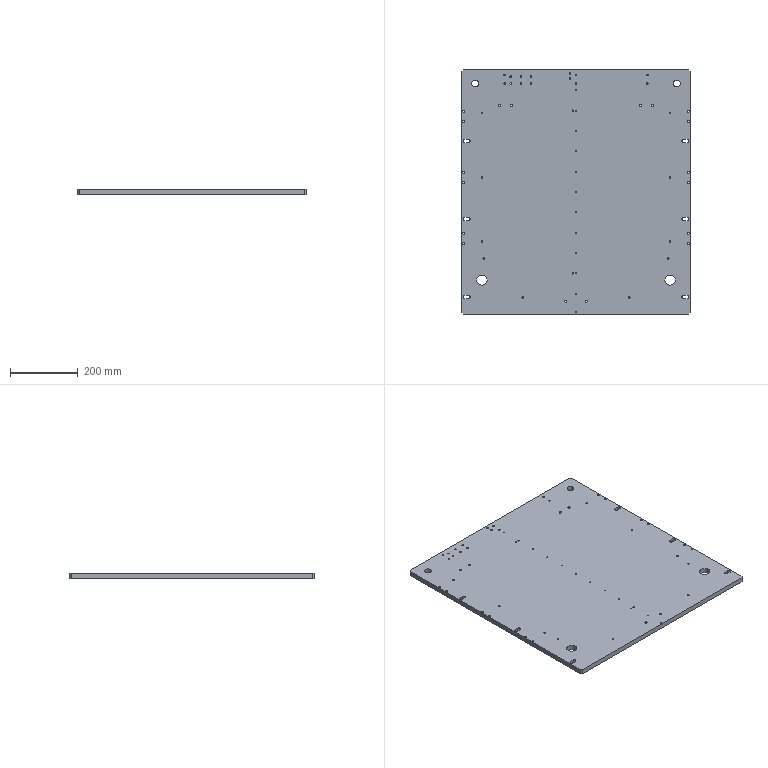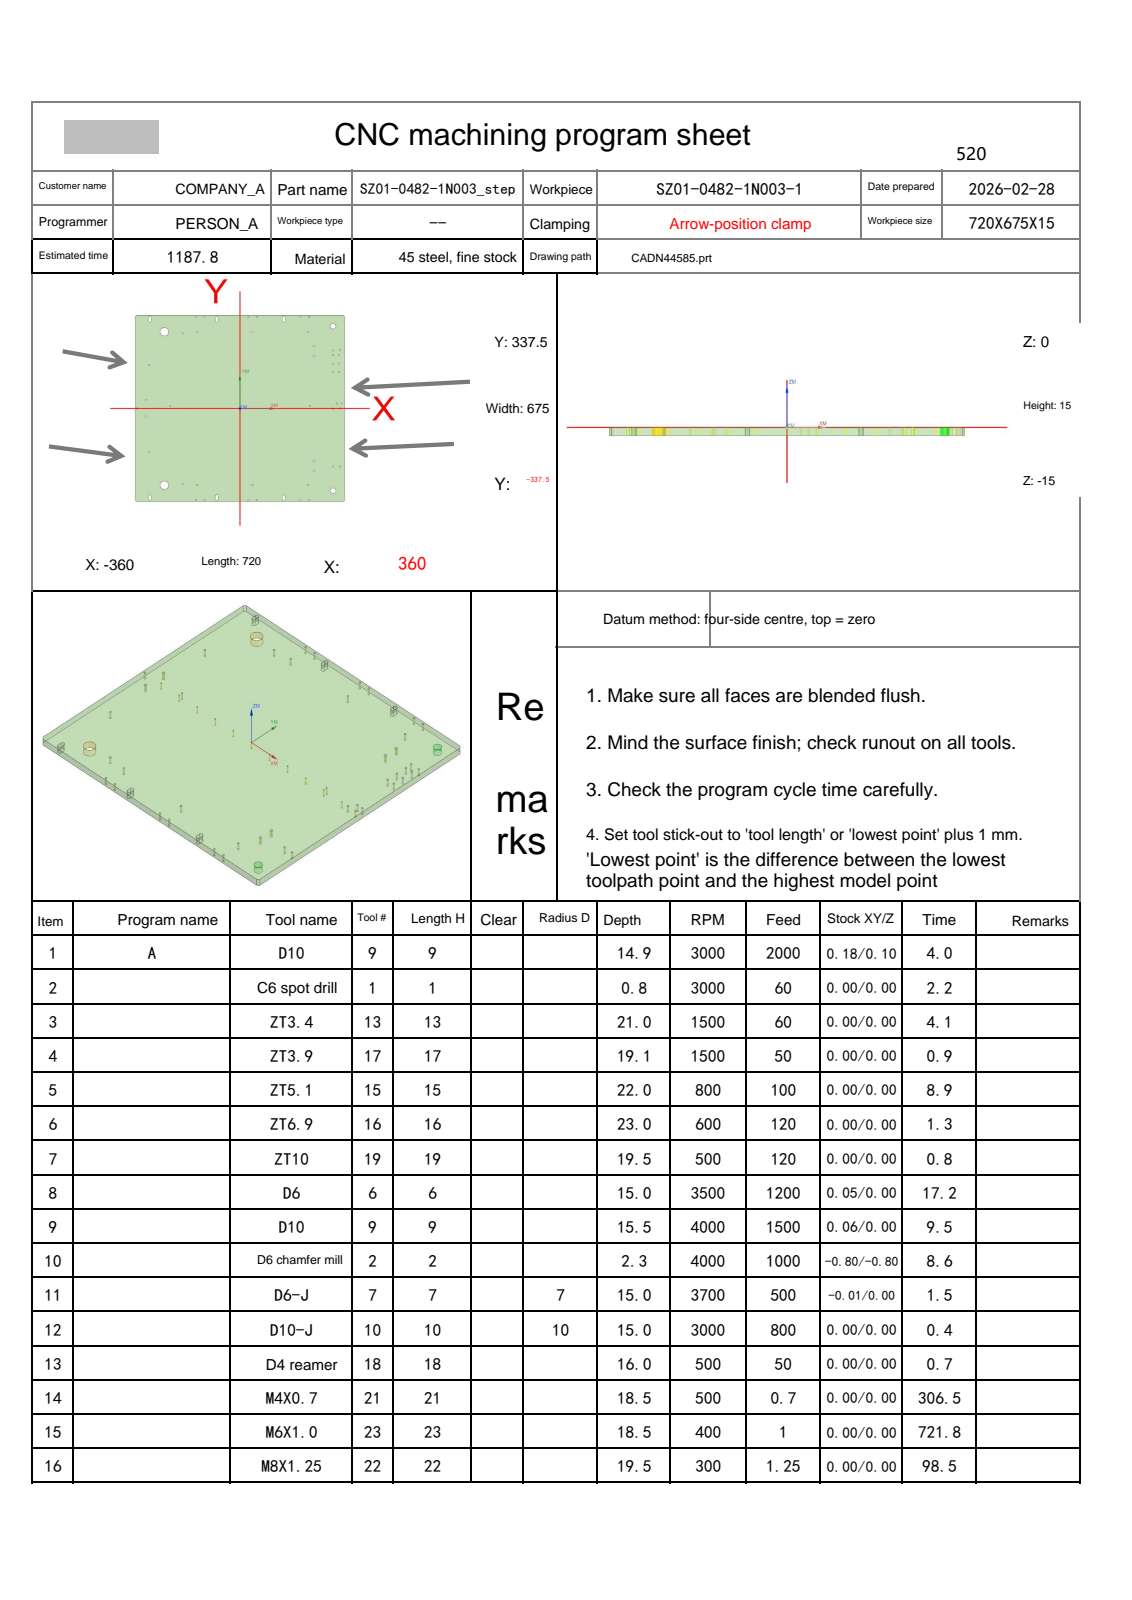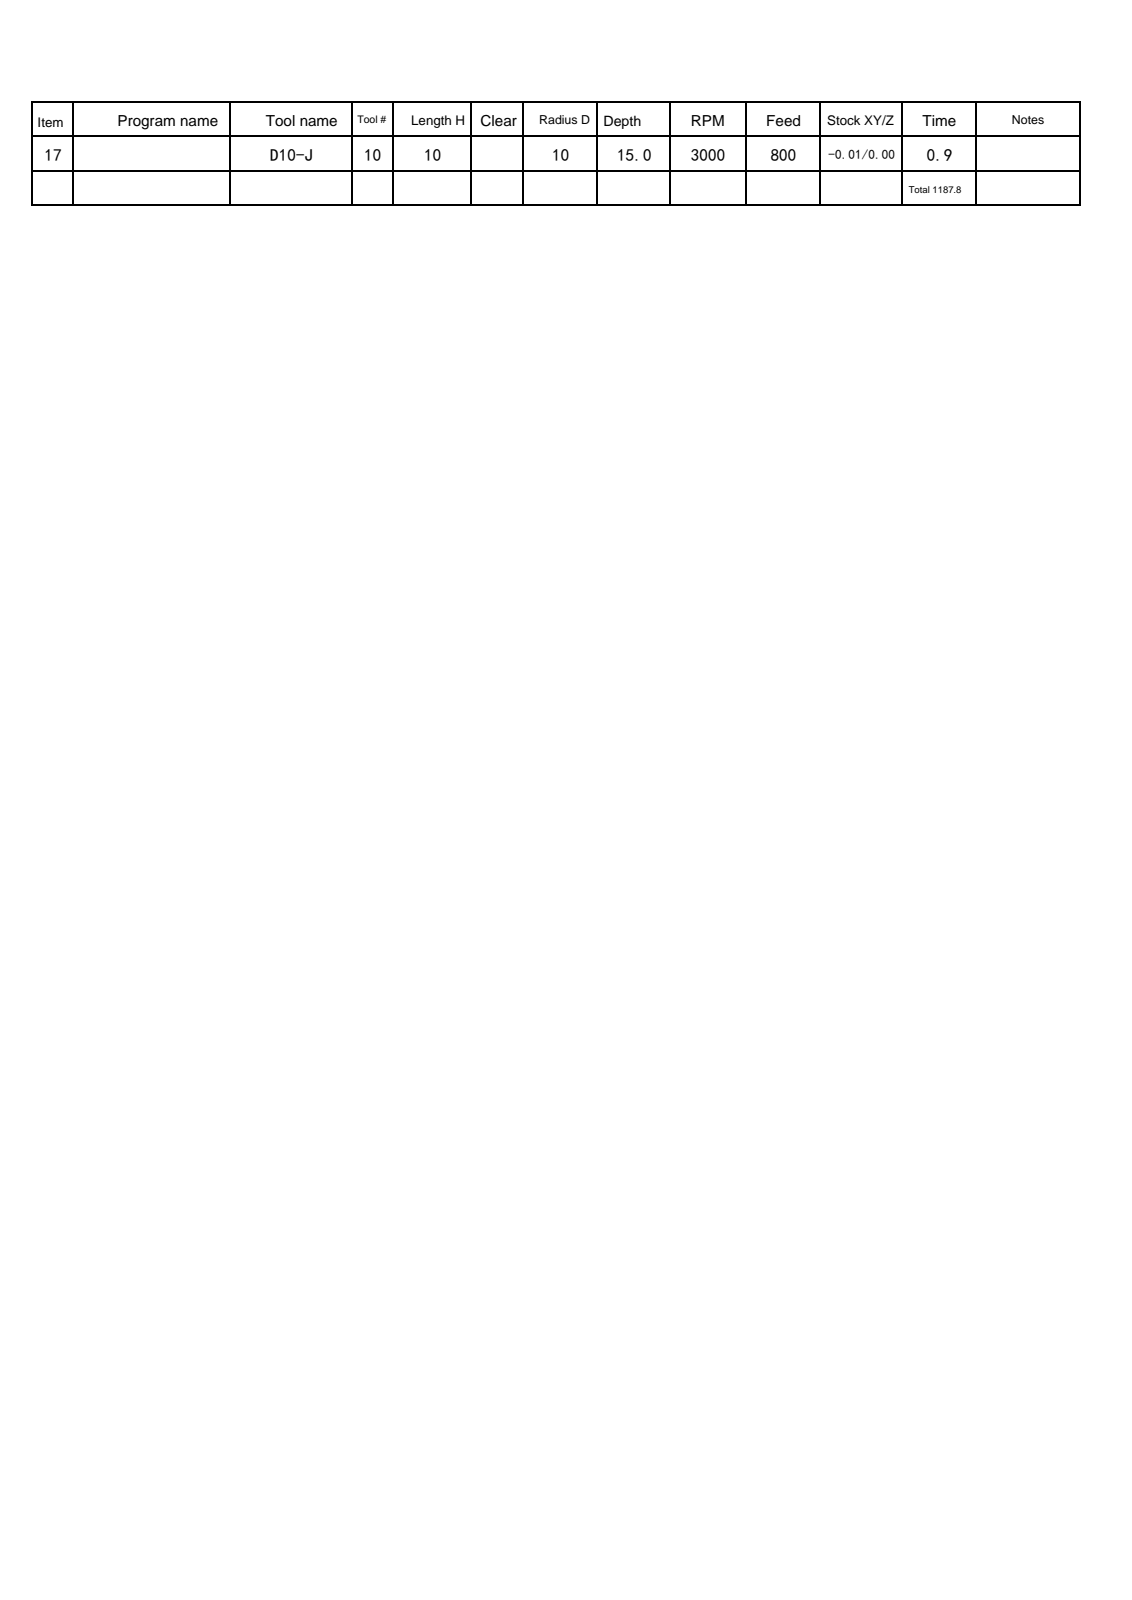NC program | NX | posted by the shop | part box 675 x 720 x 15 mm
Lines 1438 to 2224 of 7907:
N8 T06 M06
(D6  D=6. R=0. H=06 ce=0.05 di=0.00)
G00 G90 G54 X-311.95 Y322.5 M03 S3500
G43 H06 Z60.
M08
Z.5
G01 Y317.5 Z.477 F1200.
G03 X-310. Y315.55 Z.463 I1.95 J0.0
X-308.05 Y317.5 Z.449 I0.0 J1.95
G01 Y327.5 Z.402
G03 X-310. Y329.45 Z.388 I-1.95 J0.0
X-311.95 Y327.5 Z.374 I0.0 J-1.95
G01 Y317.5 Z.328
G03 X-310. Y315.55 Z.314 I1.95 J0.0
X-308.05 Y317.5 Z.3 I0.0 J1.95
G01 Y327.5 Z.253
G03 X-310. Y329.45 Z.239 I-1.95 J0.0
X-311.95 Y327.5 Z.225 I0.0 J-1.95
G01 Y317.5 Z.179
G03 X-310. Y315.55 Z.165 I1.95 J0.0
X-308.05 Y317.5 Z.151 I0.0 J1.95
G01 Y327.5 Z.104
G03 X-310. Y329.45 Z.09 I-1.95 J0.0
X-311.95 Y327.5 Z.076 I0.0 J-1.95
G01 Y317.5 Z.03
G03 X-310. Y315.55 Z.016 I1.95 J0.0
X-308.05 Y317.5 Z.001 I0.0 J1.95
G01 Y327.5 Z-.045
G03 X-310. Y329.45 Z-.059 I-1.95 J0.0
X-311.95 Y327.5 Z-.073 I0.0 J-1.95
G01 Y317.5 Z-.119
G03 X-310. Y315.55 Z-.133 I1.95 J0.0
X-308.05 Y317.5 Z-.148 I0.0 J1.95
G01 Y327.5 Z-.194
G03 X-310. Y329.45 Z-.208 I-1.95 J0.0
X-311.95 Y327.5 Z-.222 I0.0 J-1.95
G01 Y317.5 Z-.268
G03 X-310. Y315.55 Z-.282 I1.95 J0.0
X-308.05 Y317.5 Z-.297 I0.0 J1.95
G01 Y327.5 Z-.343
G03 X-310. Y329.45 Z-.357 I-1.95 J0.0
X-311.95 Y327.5 Z-.371 I0.0 J-1.95
G01 Y317.5 Z-.417
G03 X-310. Y315.55 Z-.431 I1.95 J0.0
X-308.05 Y317.5 Z-.446 I0.0 J1.95
G01 Y327.5 Z-.492
G03 X-310. Y329.45 Z-.506 I-1.95 J0.0
X-311.95 Y327.5 Z-.52 I0.0 J-1.95
G01 Y317.5 Z-.566
G03 X-310. Y315.55 Z-.581 I1.95 J0.0
X-308.05 Y317.5 Z-.595 I0.0 J1.95
G01 Y327.5 Z-.641
G03 X-310. Y329.45 Z-.655 I-1.95 J0.0
X-311.95 Y327.5 Z-.669 I0.0 J-1.95
G01 Y317.5 Z-.715
G03 X-310. Y315.55 Z-.73 I1.95 J0.0
X-308.05 Y317.5 Z-.744 I0.0 J1.95
G01 Y327.5 Z-.79
G03 X-310. Y329.45 Z-.804 I-1.95 J0.0
X-311.95 Y327.5 Z-.818 I0.0 J-1.95
G01 Y317.5 Z-.864
G03 X-310. Y315.55 Z-.879 I1.95 J0.0
X-308.05 Y317.5 Z-.893 I0.0 J1.95
G01 Y327.5 Z-.939
G03 X-310. Y329.45 Z-.953 I-1.95 J0.0
X-311.95 Y327.5 Z-.967 I0.0 J-1.95
G01 Y317.5 Z-1.013
G03 X-310. Y315.55 Z-1.028 I1.95 J0.0
X-308.05 Y317.5 Z-1.042 I0.0 J1.95
G01 Y327.5 Z-1.088
G03 X-310. Y329.45 Z-1.102 I-1.95 J0.0
X-311.95 Y327.5 Z-1.116 I0.0 J-1.95
G01 Y317.5 Z-1.163
G03 X-310. Y315.55 Z-1.177 I1.95 J0.0
X-308.05 Y317.5 Z-1.191 I0.0 J1.95
G01 Y327.5 Z-1.237
G03 X-310. Y329.45 Z-1.251 I-1.95 J0.0
X-311.95 Y327.5 Z-1.265 I0.0 J-1.95
G01 Y317.5 Z-1.312
G03 X-310. Y315.55 Z-1.326 I1.95 J0.0
X-308.05 Y317.5 Z-1.34 I0.0 J1.95
G01 Y327.5 Z-1.386
G03 X-310. Y329.45 Z-1.4 I-1.95 J0.0
X-311.95 Y327.5 Z-1.414 I0.0 J-1.95
G01 Y317.5 Z-1.461
G03 X-310. Y315.55 Z-1.475 I1.95 J0.0
X-308.05 Y317.5 Z-1.489 I0.0 J1.95
G01 Y327.5 Z-1.535
G03 X-310. Y329.45 Z-1.549 I-1.95 J0.0
X-311.95 Y327.5 Z-1.563 I0.0 J-1.95
G01 Y317.5 Z-1.61
G03 X-310. Y315.55 Z-1.624 I1.95 J0.0
X-308.05 Y317.5 Z-1.638 I0.0 J1.95
G01 Y327.5 Z-1.684
G03 X-310. Y329.45 Z-1.698 I-1.95 J0.0
X-311.95 Y327.5 Z-1.712 I0.0 J-1.95
G01 Y317.5 Z-1.759
G03 X-310. Y315.55 Z-1.773 I1.95 J0.0
X-308.05 Y317.5 Z-1.787 I0.0 J1.95
G01 Y327.5 Z-1.833
G03 X-310. Y329.45 Z-1.847 I-1.95 J0.0
X-311.95 Y327.5 Z-1.862 I0.0 J-1.95
G01 Y317.5 Z-1.908
G03 X-310. Y315.55 Z-1.922 I1.95 J0.0
X-308.05 Y317.5 Z-1.936 I0.0 J1.95
G01 Y327.5 Z-1.982
G03 X-310. Y329.45 Z-1.996 I-1.95 J0.0
X-311.95 Y327.5 Z-2.011 I0.0 J-1.95
G01 Y317.5 Z-2.057
G03 X-310. Y315.55 Z-2.071 I1.95 J0.0
X-308.05 Y317.5 Z-2.085 I0.0 J1.95
G01 Y327.5 Z-2.131
G03 X-310. Y329.45 Z-2.145 I-1.95 J0.0
X-311.95 Y327.5 Z-2.16 I0.0 J-1.95
G01 Y317.5 Z-2.206
G03 X-310. Y315.55 Z-2.22 I1.95 J0.0
X-308.05 Y317.5 Z-2.234 I0.0 J1.95
G01 Y327.5 Z-2.28
G03 X-310. Y329.45 Z-2.294 I-1.95 J0.0
X-311.95 Y327.5 Z-2.309 I0.0 J-1.95
G01 Y317.5 Z-2.355
G03 X-310. Y315.55 Z-2.369 I1.95 J0.0
X-308.05 Y317.5 Z-2.383 I0.0 J1.95
G01 Y327.5 Z-2.429
G03 X-310. Y329.45 Z-2.444 I-1.95 J0.0
X-311.95 Y327.5 Z-2.458 I0.0 J-1.95
G01 Y317.5 Z-2.504
G03 X-310. Y315.55 Z-2.518 I1.95 J0.0
X-308.05 Y317.5 Z-2.532 I0.0 J1.95
G01 Y327.5 Z-2.578
G03 X-310. Y329.45 Z-2.593 I-1.95 J0.0
X-311.95 Y327.5 Z-2.607 I0.0 J-1.95
G01 Y317.5 Z-2.653
G03 X-310. Y315.55 Z-2.667 I1.95 J0.0
X-308.05 Y317.5 Z-2.681 I0.0 J1.95
G01 Y327.5 Z-2.727
G03 X-310. Y329.45 Z-2.742 I-1.95 J0.0
X-311.95 Y327.5 Z-2.756 I0.0 J-1.95
G01 Y317.5 Z-2.802
G03 X-310. Y315.55 Z-2.816 I1.95 J0.0
X-308.05 Y317.5 Z-2.83 I0.0 J1.95
G01 Y327.5 Z-2.876
G03 X-310. Y329.45 Z-2.891 I-1.95 J0.0
X-311.95 Y327.5 Z-2.905 I0.0 J-1.95
G01 Y317.5 Z-2.951
G03 X-310. Y315.55 Z-2.965 I1.95 J0.0
X-308.05 Y317.5 Z-2.979 I0.0 J1.95
G01 Y327.5 Z-3.026
G03 X-310. Y329.45 Z-3.04 I-1.95 J0.0
X-311.95 Y327.5 Z-3.054 I0.0 J-1.95
G01 Y317.5 Z-3.1
G03 X-310. Y315.55 Z-3.114 I1.95 J0.0
X-308.05 Y317.5 Z-3.128 I0.0 J1.95
G01 Y327.5 Z-3.175
G03 X-310. Y329.45 Z-3.189 I-1.95 J0.0
X-311.95 Y327.5 Z-3.203 I0.0 J-1.95
G01 Y317.5 Z-3.249
G03 X-310. Y315.55 Z-3.263 I1.95 J0.0
X-308.05 Y317.5 Z-3.277 I0.0 J1.95
G01 Y327.5 Z-3.324
G03 X-310. Y329.45 Z-3.338 I-1.95 J0.0
X-311.95 Y327.5 Z-3.352 I0.0 J-1.95
G01 Y317.5 Z-3.398
G03 X-310. Y315.55 Z-3.412 I1.95 J0.0
X-308.05 Y317.5 Z-3.426 I0.0 J1.95
G01 Y327.5 Z-3.473
G03 X-310. Y329.45 Z-3.487 I-1.95 J0.0
X-311.95 Y327.5 Z-3.501 I0.0 J-1.95
G01 Y317.5 Z-3.547
G03 X-310. Y315.55 Z-3.561 I1.95 J0.0
X-308.05 Y317.5 Z-3.575 I0.0 J1.95
G01 Y327.5 Z-3.622
G03 X-310. Y329.45 Z-3.636 I-1.95 J0.0
X-311.95 Y327.5 Z-3.65 I0.0 J-1.95
G01 Y317.5 Z-3.696
G03 X-310. Y315.55 Z-3.71 I1.95 J0.0
X-308.05 Y317.5 Z-3.724 I0.0 J1.95
G01 Y327.5 Z-3.771
G03 X-310. Y329.45 Z-3.785 I-1.95 J0.0
X-311.95 Y327.5 Z-3.799 I0.0 J-1.95
G01 Y317.5 Z-3.845
G03 X-310. Y315.55 Z-3.859 I1.95 J0.0
X-308.05 Y317.5 Z-3.874 I0.0 J1.95
G01 Y327.5 Z-3.92
G03 X-310. Y329.45 Z-3.934 I-1.95 J0.0
X-311.95 Y327.5 Z-3.948 I0.0 J-1.95
G01 Y317.5 Z-3.994
G03 X-310. Y315.55 Z-4.008 I1.95 J0.0
X-308.05 Y317.5 Z-4.023 I0.0 J1.95
G01 Y327.5 Z-4.069
G03 X-310. Y329.45 Z-4.083 I-1.95 J0.0
X-311.95 Y327.5 Z-4.097 I0.0 J-1.95
G01 Y317.5 Z-4.143
G03 X-310. Y315.55 Z-4.157 I1.95 J0.0
X-308.05 Y317.5 Z-4.172 I0.0 J1.95
G01 Y327.5 Z-4.218
G03 X-310. Y329.45 Z-4.232 I-1.95 J0.0
X-311.95 Y327.5 Z-4.246 I0.0 J-1.95
G01 Y317.5 Z-4.292
G03 X-310. Y315.55 Z-4.306 I1.95 J0.0
X-308.05 Y317.5 Z-4.321 I0.0 J1.95
G01 Y327.5 Z-4.367
G03 X-310. Y329.45 Z-4.381 I-1.95 J0.0
X-311.95 Y327.5 Z-4.395 I0.0 J-1.95
G01 Y317.5 Z-4.441
G03 X-310. Y315.55 Z-4.456 I1.95 J0.0
X-308.05 Y317.5 Z-4.47 I0.0 J1.95
G01 Y327.5 Z-4.516
G03 X-310. Y329.45 Z-4.53 I-1.95 J0.0
X-311.95 Y327.5 Z-4.544 I0.0 J-1.95
G01 Y317.5 Z-4.59
G03 X-310. Y315.55 Z-4.605 I1.95 J0.0
X-308.05 Y317.5 Z-4.619 I0.0 J1.95
G01 Y327.5 Z-4.665
G03 X-310. Y329.45 Z-4.679 I-1.95 J0.0
X-311.95 Y327.5 Z-4.693 I0.0 J-1.95
G01 Y317.5 Z-4.739
G03 X-310. Y315.55 Z-4.754 I1.95 J0.0
X-308.05 Y317.5 Z-4.768 I0.0 J1.95
G01 Y327.5 Z-4.814
G03 X-310. Y329.45 Z-4.828 I-1.95 J0.0
X-311.95 Y327.5 Z-4.842 I0.0 J-1.95
G01 Y317.5 Z-4.888
G03 X-310. Y315.55 Z-4.903 I1.95 J0.0
X-308.05 Y317.5 Z-4.917 I0.0 J1.95
G01 Y327.5 Z-4.963
G03 X-310. Y329.45 Z-4.977 I-1.95 J0.0
X-311.95 Y327.5 Z-4.991 I0.0 J-1.95
G01 Y317.5 Z-5.038
G03 X-310. Y315.55 Z-5.052 I1.95 J0.0
X-308.05 Y317.5 Z-5.066 I0.0 J1.95
G01 Y327.5 Z-5.112
G03 X-310. Y329.45 Z-5.126 I-1.95 J0.0
X-311.95 Y327.5 Z-5.14 I0.0 J-1.95
G01 Y317.5 Z-5.187
G03 X-310. Y315.55 Z-5.201 I1.95 J0.0
X-308.05 Y317.5 Z-5.215 I0.0 J1.95
G01 Y327.5 Z-5.261
G03 X-310. Y329.45 Z-5.275 I-1.95 J0.0
X-311.95 Y327.5 Z-5.289 I0.0 J-1.95
G01 Y317.5 Z-5.336
G03 X-310. Y315.55 Z-5.35 I1.95 J0.0
X-308.05 Y317.5 Z-5.364 I0.0 J1.95
G01 Y327.5 Z-5.41
G03 X-310. Y329.45 Z-5.424 I-1.95 J0.0
X-311.95 Y327.5 Z-5.438 I0.0 J-1.95
G01 Y317.5 Z-5.485
G03 X-310. Y315.55 Z-5.499 I1.95 J0.0
X-308.05 Y317.5 Z-5.513 I0.0 J1.95
G01 Y327.5 Z-5.559
G03 X-310. Y329.45 Z-5.573 I-1.95 J0.0
X-311.95 Y327.5 Z-5.587 I0.0 J-1.95
G01 Y317.5 Z-5.634
G03 X-310. Y315.55 Z-5.648 I1.95 J0.0
X-308.05 Y317.5 Z-5.662 I0.0 J1.95
G01 Y327.5 Z-5.708
G03 X-310. Y329.45 Z-5.722 I-1.95 J0.0
X-311.95 Y327.5 Z-5.737 I0.0 J-1.95
G01 Y317.5 Z-5.783
G03 X-310. Y315.55 Z-5.797 I1.95 J0.0
X-308.05 Y317.5 Z-5.811 I0.0 J1.95
G01 Y327.5 Z-5.857
G03 X-310. Y329.45 Z-5.871 I-1.95 J0.0
X-311.95 Y327.5 Z-5.886 I0.0 J-1.95
G01 Y317.5 Z-5.932
G03 X-310. Y315.55 Z-5.946 I1.95 J0.0
X-308.05 Y317.5 Z-5.96 I0.0 J1.95
G01 Y327.5 Z-6.006
G03 X-310. Y329.45 Z-6.02 I-1.95 J0.0
X-311.95 Y327.5 Z-6.035 I0.0 J-1.95
G01 Y317.5 Z-6.081
G03 X-310. Y315.55 Z-6.095 I1.95 J0.0
X-308.05 Y317.5 Z-6.109 I0.0 J1.95
G01 Y327.5 Z-6.155
G03 X-310. Y329.45 Z-6.169 I-1.95 J0.0
X-311.95 Y327.5 Z-6.184 I0.0 J-1.95
G01 Y317.5 Z-6.23
G03 X-310. Y315.55 Z-6.244 I1.95 J0.0
X-308.05 Y317.5 Z-6.258 I0.0 J1.95
G01 Y327.5 Z-6.304
G03 X-310. Y329.45 Z-6.319 I-1.95 J0.0
X-311.95 Y327.5 Z-6.333 I0.0 J-1.95
G01 Y317.5 Z-6.379
G03 X-310. Y315.55 Z-6.393 I1.95 J0.0
X-308.05 Y317.5 Z-6.407 I0.0 J1.95
G01 Y327.5 Z-6.453
G03 X-310. Y329.45 Z-6.468 I-1.95 J0.0
X-311.95 Y327.5 Z-6.482 I0.0 J-1.95
G01 Y317.5 Z-6.528
G03 X-310. Y315.55 Z-6.542 I1.95 J0.0
X-308.05 Y317.5 Z-6.556 I0.0 J1.95
G01 Y327.5 Z-6.602
G03 X-310. Y329.45 Z-6.617 I-1.95 J0.0
X-311.95 Y327.5 Z-6.631 I0.0 J-1.95
G01 Y317.5 Z-6.677
G03 X-310. Y315.55 Z-6.691 I1.95 J0.0
X-308.05 Y317.5 Z-6.705 I0.0 J1.95
G01 Y327.5 Z-6.751
G03 X-310. Y329.45 Z-6.766 I-1.95 J0.0
X-311.95 Y327.5 Z-6.78 I0.0 J-1.95
G01 Y317.5 Z-6.826
G03 X-310. Y315.55 Z-6.84 I1.95 J0.0
X-308.05 Y317.5 Z-6.854 I0.0 J1.95
G01 Y327.5 Z-6.901
G03 X-310. Y329.45 Z-6.915 I-1.95 J0.0
X-311.95 Y327.5 Z-6.929 I0.0 J-1.95
G01 Y317.5 Z-6.975
G03 X-310. Y315.55 Z-6.989 I1.95 J0.0
X-308.05 Y317.5 Z-7.003 I0.0 J1.95
G01 Y327.5 Z-7.05
G03 X-310. Y329.45 Z-7.064 I-1.95 J0.0
X-311.95 Y327.5 Z-7.078 I0.0 J-1.95
G01 Y317.5 Z-7.124
G03 X-310. Y315.55 Z-7.138 I1.95 J0.0
X-308.05 Y317.5 Z-7.152 I0.0 J1.95
G01 Y327.5 Z-7.199
G03 X-310. Y329.45 Z-7.213 I-1.95 J0.0
X-311.95 Y327.5 Z-7.227 I0.0 J-1.95
G01 Y317.5 Z-7.273
G03 X-310. Y315.55 Z-7.287 I1.95 J0.0
X-308.05 Y317.5 Z-7.301 I0.0 J1.95
G01 Y327.5 Z-7.348
G03 X-310. Y329.45 Z-7.362 I-1.95 J0.0
X-311.95 Y327.5 Z-7.376 I0.0 J-1.95
G01 Y317.5 Z-7.422
G03 X-310. Y315.55 Z-7.436 I1.95 J0.0
X-308.05 Y317.5 Z-7.45 I0.0 J1.95
G01 Y327.5 Z-7.497
G03 X-310. Y329.45 Z-7.511 I-1.95 J0.0
X-311.95 Y327.5 Z-7.525 I0.0 J-1.95
G01 Y317.5 Z-7.571
G03 X-310. Y315.55 Z-7.585 I1.95 J0.0
X-308.05 Y317.5 Z-7.599 I0.0 J1.95
G01 Y327.5 Z-7.646
G03 X-310. Y329.45 Z-7.66 I-1.95 J0.0
X-311.95 Y327.5 Z-7.674 I0.0 J-1.95
G01 Y317.5 Z-7.72
G03 X-310. Y315.55 Z-7.734 I1.95 J0.0
X-308.05 Y317.5 Z-7.749 I0.0 J1.95
G01 Y327.5 Z-7.795
G03 X-310. Y329.45 Z-7.809 I-1.95 J0.0
X-311.95 Y327.5 Z-7.823 I0.0 J-1.95
G01 Y317.5 Z-7.869
G03 X-310. Y315.55 Z-7.883 I1.95 J0.0
X-308.05 Y317.5 Z-7.898 I0.0 J1.95
G01 Y327.5 Z-7.944
G03 X-310. Y329.45 Z-7.958 I-1.95 J0.0
X-311.95 Y327.5 Z-7.972 I0.0 J-1.95
G01 Y317.5 Z-8.018
G03 X-310. Y315.55 Z-8.032 I1.95 J0.0
X-308.05 Y317.5 Z-8.047 I0.0 J1.95
G01 Y327.5 Z-8.093
G03 X-310. Y329.45 Z-8.107 I-1.95 J0.0
X-311.95 Y327.5 Z-8.121 I0.0 J-1.95
G01 Y317.5 Z-8.167
G03 X-310. Y315.55 Z-8.181 I1.95 J0.0
X-308.05 Y317.5 Z-8.196 I0.0 J1.95
G01 Y327.5 Z-8.242
G03 X-310. Y329.45 Z-8.256 I-1.95 J0.0
X-311.95 Y327.5 Z-8.27 I0.0 J-1.95
G01 Y317.5 Z-8.316
G03 X-310. Y315.55 Z-8.331 I1.95 J0.0
X-308.05 Y317.5 Z-8.345 I0.0 J1.95
G01 Y327.5 Z-8.391
G03 X-310. Y329.45 Z-8.405 I-1.95 J0.0
X-311.95 Y327.5 Z-8.419 I0.0 J-1.95
G01 Y317.5 Z-8.465
G03 X-310. Y315.55 Z-8.48 I1.95 J0.0
X-308.05 Y317.5 Z-8.494 I0.0 J1.95
G01 Y327.5 Z-8.54
G03 X-310. Y329.45 Z-8.554 I-1.95 J0.0
X-311.95 Y327.5 Z-8.568 I0.0 J-1.95
G01 Y317.5 Z-8.614
G03 X-310. Y315.55 Z-8.629 I1.95 J0.0
X-308.05 Y317.5 Z-8.643 I0.0 J1.95
G01 Y327.5 Z-8.689
G03 X-310. Y329.45 Z-8.703 I-1.95 J0.0
X-311.95 Y327.5 Z-8.717 I0.0 J-1.95
G01 Y317.5 Z-8.763
G03 X-310. Y315.55 Z-8.778 I1.95 J0.0
X-308.05 Y317.5 Z-8.792 I0.0 J1.95
G01 Y327.5 Z-8.838
G03 X-310. Y329.45 Z-8.852 I-1.95 J0.0
X-311.95 Y327.5 Z-8.866 I0.0 J-1.95
G01 Y317.5 Z-8.913
G03 X-310. Y315.55 Z-8.927 I1.95 J0.0
X-308.05 Y317.5 Z-8.941 I0.0 J1.95
G01 Y327.5 Z-8.987
G03 X-310. Y329.45 Z-9.001 I-1.95 J0.0
X-311.95 Y327.5 Z-9.015 I0.0 J-1.95
G01 Y317.5 Z-9.062
G03 X-310. Y315.55 Z-9.076 I1.95 J0.0
X-308.05 Y317.5 Z-9.09 I0.0 J1.95
G01 Y327.5 Z-9.136
G03 X-310. Y329.45 Z-9.15 I-1.95 J0.0
X-311.95 Y327.5 Z-9.164 I0.0 J-1.95
G01 Y317.5 Z-9.211
G03 X-310. Y315.55 Z-9.225 I1.95 J0.0
X-308.05 Y317.5 Z-9.239 I0.0 J1.95
G01 Y327.5 Z-9.285
G03 X-310. Y329.45 Z-9.299 I-1.95 J0.0
X-311.95 Y327.5 Z-9.313 I0.0 J-1.95
G01 Y317.5 Z-9.36
G03 X-310. Y315.55 Z-9.374 I1.95 J0.0
X-308.05 Y317.5 Z-9.388 I0.0 J1.95
G01 Y327.5 Z-9.434
G03 X-310. Y329.45 Z-9.448 I-1.95 J0.0
X-311.95 Y327.5 Z-9.462 I0.0 J-1.95
G01 Y317.5 Z-9.509
G03 X-310. Y315.55 Z-9.523 I1.95 J0.0
X-308.05 Y317.5 Z-9.537 I0.0 J1.95
G01 Y327.5 Z-9.583
G03 X-310. Y329.45 Z-9.597 I-1.95 J0.0
X-311.95 Y327.5 Z-9.612 I0.0 J-1.95
G01 Y317.5 Z-9.658
G03 X-310. Y315.55 Z-9.672 I1.95 J0.0
X-308.05 Y317.5 Z-9.686 I0.0 J1.95
G01 Y327.5 Z-9.732
G03 X-310. Y329.45 Z-9.746 I-1.95 J0.0
X-311.95 Y327.5 Z-9.761 I0.0 J-1.95
G01 Y317.5 Z-9.807
G03 X-310. Y315.55 Z-9.821 I1.95 J0.0
X-308.05 Y317.5 Z-9.835 I0.0 J1.95
G01 Y327.5 Z-9.881
G03 X-310. Y329.45 Z-9.895 I-1.95 J0.0
X-311.95 Y327.5 Z-9.91 I0.0 J-1.95
G01 Y317.5 Z-9.956
G03 X-310. Y315.55 Z-9.97 I1.95 J0.0
X-308.05 Y317.5 Z-9.984 I0.0 J1.95
G01 Y327.5 Z-10.03
G03 X-310. Y329.45 Z-10.044 I-1.95 J0.0
X-311.95 Y327.5 Z-10.059 I0.0 J-1.95
G01 Y317.5 Z-10.105
G03 X-310. Y315.55 Z-10.119 I1.95 J0.0
X-308.05 Y317.5 Z-10.133 I0.0 J1.95
G01 Y327.5 Z-10.179
G03 X-310. Y329.45 Z-10.194 I-1.95 J0.0
X-311.95 Y327.5 Z-10.208 I0.0 J-1.95
G01 Y317.5 Z-10.254
G03 X-310. Y315.55 Z-10.268 I1.95 J0.0
X-308.05 Y317.5 Z-10.282 I0.0 J1.95
G01 Y327.5 Z-10.328
G03 X-310. Y329.45 Z-10.343 I-1.95 J0.0
X-311.95 Y327.5 Z-10.357 I0.0 J-1.95
G01 Y317.5 Z-10.403
G03 X-310. Y315.55 Z-10.417 I1.95 J0.0
X-308.05 Y317.5 Z-10.431 I0.0 J1.95
G01 Y327.5 Z-10.477
G03 X-310. Y329.45 Z-10.492 I-1.95 J0.0
X-311.95 Y327.5 Z-10.506 I0.0 J-1.95
G01 Y317.5 Z-10.552
G03 X-310. Y315.55 Z-10.566 I1.95 J0.0
X-308.05 Y317.5 Z-10.58 I0.0 J1.95
G01 Y327.5 Z-10.626
G03 X-310. Y329.45 Z-10.641 I-1.95 J0.0
X-311.95 Y327.5 Z-10.655 I0.0 J-1.95
G01 Y317.5 Z-10.701
G03 X-310. Y315.55 Z-10.715 I1.95 J0.0
X-308.05 Y317.5 Z-10.729 I0.0 J1.95
G01 Y327.5 Z-10.776
G03 X-310. Y329.45 Z-10.79 I-1.95 J0.0
X-311.95 Y327.5 Z-10.804 I0.0 J-1.95
G01 Y317.5 Z-10.85
G03 X-310. Y315.55 Z-10.864 I1.95 J0.0
X-308.05 Y317.5 Z-10.878 I0.0 J1.95
G01 Y327.5 Z-10.925
G03 X-310. Y329.45 Z-10.939 I-1.95 J0.0
X-311.95 Y327.5 Z-10.953 I0.0 J-1.95
G01 Y317.5 Z-10.999
G03 X-310. Y315.55 Z-11.013 I1.95 J0.0
X-308.05 Y317.5 Z-11.027 I0.0 J1.95
G01 Y327.5 Z-11.074
G03 X-310. Y329.45 Z-11.088 I-1.95 J0.0
X-311.95 Y327.5 Z-11.102 I0.0 J-1.95
G01 Y317.5 Z-11.148
G03 X-310. Y315.55 Z-11.162 I1.95 J0.0
X-308.05 Y317.5 Z-11.176 I0.0 J1.95
G01 Y327.5 Z-11.223
G03 X-310. Y329.45 Z-11.237 I-1.95 J0.0
X-311.95 Y327.5 Z-11.251 I0.0 J-1.95
G01 Y317.5 Z-11.297
G03 X-310. Y315.55 Z-11.311 I1.95 J0.0
X-308.05 Y317.5 Z-11.325 I0.0 J1.95
G01 Y327.5 Z-11.372
G03 X-310. Y329.45 Z-11.386 I-1.95 J0.0
X-311.95 Y327.5 Z-11.4 I0.0 J-1.95
G01 Y317.5 Z-11.446
G03 X-310. Y315.55 Z-11.46 I1.95 J0.0
X-308.05 Y317.5 Z-11.474 I0.0 J1.95
G01 Y327.5 Z-11.521
G03 X-310. Y329.45 Z-11.535 I-1.95 J0.0
X-311.95 Y327.5 Z-11.549 I0.0 J-1.95
G01 Y317.5 Z-11.595
G03 X-310. Y315.55 Z-11.609 I1.95 J0.0
X-308.05 Y317.5 Z-11.624 I0.0 J1.95
G01 Y327.5 Z-11.67
G03 X-310. Y329.45 Z-11.684 I-1.95 J0.0
X-311.95 Y327.5 Z-11.698 I0.0 J-1.95
G01 Y317.5 Z-11.744
G03 X-310. Y315.55 Z-11.758 I1.95 J0.0
X-308.05 Y317.5 Z-11.773 I0.0 J1.95
G01 Y327.5 Z-11.819
G03 X-310. Y329.45 Z-11.833 I-1.95 J0.0
X-311.95 Y327.5 Z-11.847 I0.0 J-1.95
G01 Y317.5 Z-11.893
G03 X-310. Y315.55 Z-11.907 I1.95 J0.0
X-308.05 Y317.5 Z-11.922 I0.0 J1.95
G01 Y327.5 Z-11.968
G03 X-310. Y329.45 Z-11.982 I-1.95 J0.0
X-311.95 Y327.5 Z-11.996 I0.0 J-1.95
G01 Y317.5 Z-12.042
G03 X-310. Y315.55 Z-12.056 I1.95 J0.0
X-308.05 Y317.5 Z-12.071 I0.0 J1.95
G01 Y327.5 Z-12.117
G03 X-310. Y329.45 Z-12.131 I-1.95 J0.0
X-311.95 Y327.5 Z-12.145 I0.0 J-1.95
G01 Y317.5 Z-12.191
G03 X-310. Y315.55 Z-12.206 I1.95 J0.0
X-308.05 Y317.5 Z-12.22 I0.0 J1.95
G01 Y327.5 Z-12.266
G03 X-310. Y329.45 Z-12.28 I-1.95 J0.0
X-311.95 Y327.5 Z-12.294 I0.0 J-1.95
G01 Y317.5 Z-12.34
G03 X-310. Y315.55 Z-12.355 I1.95 J0.0
X-308.05 Y317.5 Z-12.369 I0.0 J1.95
G01 Y327.5 Z-12.415
G03 X-310. Y329.45 Z-12.429 I-1.95 J0.0
X-311.95 Y327.5 Z-12.443 I0.0 J-1.95
G01 Y317.5 Z-12.489
G03 X-310. Y315.55 Z-12.504 I1.95 J0.0
X-308.05 Y317.5 Z-12.518 I0.0 J1.95
G01 Y327.5 Z-12.564
G03 X-310. Y329.45 Z-12.578 I-1.95 J0.0
X-311.95 Y327.5 Z-12.592 I0.0 J-1.95
G01 Y317.5 Z-12.638
G03 X-310. Y315.55 Z-12.653 I1.95 J0.0
X-308.05 Y317.5 Z-12.667 I0.0 J1.95
G01 Y327.5 Z-12.713
G03 X-310. Y329.45 Z-12.727 I-1.95 J0.0
X-311.95 Y327.5 Z-12.741 I0.0 J-1.95
G01 Y317.5 Z-12.788
G03 X-310. Y315.55 Z-12.802 I1.95 J0.0
X-308.05 Y317.5 Z-12.816 I0.0 J1.95
G01 Y327.5 Z-12.862
G03 X-310. Y329.45 Z-12.876 I-1.95 J0.0
X-311.95 Y327.5 Z-12.89 I0.0 J-1.95
G01 Y317.5 Z-12.937
G03 X-310. Y315.55 Z-12.951 I1.95 J0.0
X-308.05 Y317.5 Z-12.965 I0.0 J1.95
G01 Y327.5 Z-13.011
G03 X-310. Y329.45 Z-13.025 I-1.95 J0.0
X-311.95 Y327.5 Z-13.039 I0.0 J-1.95
G01 Y317.5 Z-13.086
G03 X-310. Y315.55 Z-13.1 I1.95 J0.0
X-308.05 Y317.5 Z-13.114 I0.0 J1.95
G01 Y327.5 Z-13.16
G03 X-310. Y329.45 Z-13.174 I-1.95 J0.0
X-311.95 Y327.5 Z-13.188 I0.0 J-1.95
G01 Y317.5 Z-13.235
G03 X-310. Y315.55 Z-13.249 I1.95 J0.0
X-308.05 Y317.5 Z-13.263 I0.0 J1.95
G01 Y327.5 Z-13.309
G03 X-310. Y329.45 Z-13.323 I-1.95 J0.0
X-311.95 Y327.5 Z-13.337 I0.0 J-1.95
G01 Y317.5 Z-13.384
G03 X-310. Y315.55 Z-13.398 I1.95 J0.0
X-308.05 Y317.5 Z-13.412 I0.0 J1.95
G01 Y327.5 Z-13.458
G03 X-310. Y329.45 Z-13.472 I-1.95 J0.0
X-311.95 Y327.5 Z-13.487 I0.0 J-1.95
G01 Y317.5 Z-13.533
G03 X-310. Y315.55 Z-13.547 I1.95 J0.0
X-308.05 Y317.5 Z-13.561 I0.0 J1.95
G01 Y327.5 Z-13.607
G03 X-310. Y329.45 Z-13.621 I-1.95 J0.0
X-311.95 Y327.5 Z-13.636 I0.0 J-1.95
G01 Y317.5 Z-13.682
G03 X-310. Y315.55 Z-13.696 I1.95 J0.0
X-308.05 Y317.5 Z-13.71 I0.0 J1.95
G01 Y327.5 Z-13.756
G03 X-310. Y329.45 Z-13.77 I-1.95 J0.0
X-311.95 Y327.5 Z-13.785 I0.0 J-1.95
G01 Y317.5 Z-13.831
G03 X-310. Y315.55 Z-13.845 I1.95 J0.0
X-308.05 Y317.5 Z-13.859 I0.0 J1.95
G01 Y327.5 Z-13.905
G03 X-310. Y329.45 Z-13.919 I-1.95 J0.0
X-311.95 Y327.5 Z-13.934 I0.0 J-1.95
G01 Y317.5 Z-13.98
G03 X-310. Y315.55 Z-13.994 I1.95 J0.0
X-308.05 Y317.5 Z-14.008 I0.0 J1.95
G01 Y327.5 Z-14.054
G03 X-310. Y329.45 Z-14.069 I-1.95 J0.0
X-311.95 Y327.5 Z-14.083 I0.0 J-1.95
G01 Y317.5 Z-14.129
G03 X-310. Y315.55 Z-14.143 I1.95 J0.0
X-308.05 Y317.5 Z-14.157 I0.0 J1.95
G01 Y327.5 Z-14.203
G03 X-310. Y329.45 Z-14.218 I-1.95 J0.0
X-311.95 Y327.5 Z-14.232 I0.0 J-1.95
G01 Y317.5 Z-14.278
G03 X-310. Y315.55 Z-14.292 I1.95 J0.0
X-308.05 Y317.5 Z-14.306 I0.0 J1.95
G01 Y327.5 Z-14.352
G03 X-310. Y329.45 Z-14.367 I-1.95 J0.0
X-311.95 Y327.5 Z-14.381 I0.0 J-1.95
G01 Y317.5 Z-14.427
G03 X-310. Y315.55 Z-14.441 I1.95 J0.0
X-308.05 Y317.5 Z-14.455 I0.0 J1.95
G01 Y327.5 Z-14.501
G03 X-310. Y329.45 Z-14.516 I-1.95 J0.0
X-311.95 Y327.5 Z-14.53 I0.0 J-1.95
G01 Y317.5 Z-14.576
G03 X-310. Y315.55 Z-14.59 I1.95 J0.0
X-308.05 Y317.5 Z-14.604 I0.0 J1.95
G01 Y327.5 Z-14.651
G03 X-310. Y329.45 Z-14.665 I-1.95 J0.0
X-311.95 Y327.5 Z-14.679 I0.0 J-1.95
G01 Y317.5 Z-14.725
G03 X-310. Y315.55 Z-14.739 I1.95 J0.0
X-308.05 Y317.5 Z-14.753 I0.0 J1.95
G01 Y327.5 Z-14.8
G03 X-310. Y329.45 Z-14.814 I-1.95 J0.0
X-311.95 Y327.5 Z-14.828 I0.0 J-1.95
G01 Y317.5 Z-14.874
G03 X-310. Y315.55 Z-14.888 I1.95 J0.0
X-308.05 Y317.5 Z-14.902 I0.0 J1.95
G01 Y327.5 Z-14.949
G03 X-310. Y329.45 Z-14.963 I-1.95 J0.0
X-311.95 Y327.5 Z-14.977 I0.0 J-1.95
G01 Y322.5 Z-15.
Y317.5
G03 X-310. Y315.55 I1.95 J0.0
X-308.05 Y317.5 I0.0 J1.95
G01 Y327.5
G03 X-310. Y329.45 I-1.95 J0.0
X-311.95 Y327.5 I0.0 J-1.95
G01 Y322.5
Y322.
Z-14.
G00 Z60.
X-81.95 Y322.5
Z.5
G01 Y317.5 Z.477
G03 X-80. Y315.55 Z.463 I1.95 J0.0
X-78.05 Y317.5 Z.449 I0.0 J1.95
G01 Y327.5 Z.402
G03 X-80. Y329.45 Z.388 I-1.95 J0.0
X-81.95 Y327.5 Z.374 I0.0 J-1.95
G01 Y317.5 Z.328
G03 X-80. Y315.55 Z.314 I1.95 J0.0
X-78.05 Y317.5 Z.3 I0.0 J1.95
G01 Y327.5 Z.253
G03 X-80. Y329.45 Z.239 I-1.95 J0.0
X-81.95 Y327.5 Z.225 I0.0 J-1.95
G01 Y317.5 Z.179
G03 X-80. Y315.55 Z.165 I1.95 J0.0
X-78.05 Y317.5 Z.151 I0.0 J1.95
G01 Y327.5 Z.104
G03 X-80. Y329.45 Z.09 I-1.95 J0.0
X-81.95 Y327.5 Z.076 I0.0 J-1.95
G01 Y317.5 Z.03
G03 X-80. Y315.55 Z.016 I1.95 J0.0
X-78.05 Y317.5 Z.001 I0.0 J1.95
G01 Y327.5 Z-.045
G03 X-80. Y329.45 Z-.059 I-1.95 J0.0
X-81.95 Y327.5 Z-.073 I0.0 J-1.95
G01 Y317.5 Z-.119
G03 X-80. Y315.55 Z-.133 I1.95 J0.0
X-78.05 Y317.5 Z-.148 I0.0 J1.95
G01 Y327.5 Z-.194
G03 X-80. Y329.45 Z-.208 I-1.95 J0.0
X-81.95 Y327.5 Z-.222 I0.0 J-1.95
G01 Y317.5 Z-.268
G03 X-80. Y315.55 Z-.282 I1.95 J0.0
X-78.05 Y317.5 Z-.297 I0.0 J1.95
G01 Y327.5 Z-.343
G03 X-80. Y329.45 Z-.357 I-1.95 J0.0
X-81.95 Y327.5 Z-.371 I0.0 J-1.95
G01 Y317.5 Z-.417
G03 X-80. Y315.55 Z-.431 I1.95 J0.0
X-78.05 Y317.5 Z-.446 I0.0 J1.95
G01 Y327.5 Z-.492
G03 X-80. Y329.45 Z-.506 I-1.95 J0.0
X-81.95 Y327.5 Z-.52 I0.0 J-1.95
G01 Y317.5 Z-.566
G03 X-80. Y315.55 Z-.581 I1.95 J0.0
X-78.05 Y317.5 Z-.595 I0.0 J1.95
G01 Y327.5 Z-.641
G03 X-80. Y329.45 Z-.655 I-1.95 J0.0
X-81.95 Y327.5 Z-.669 I0.0 J-1.95
G01 Y317.5 Z-.715
G03 X-80. Y315.55 Z-.73 I1.95 J0.0
X-78.05 Y317.5 Z-.744 I0.0 J1.95
G01 Y327.5 Z-.79
G03 X-80. Y329.45 Z-.804 I-1.95 J0.0
X-81.95 Y327.5 Z-.818 I0.0 J-1.95
G01 Y317.5 Z-.864
G03 X-80. Y315.55 Z-.879 I1.95 J0.0
X-78.05 Y317.5 Z-.893 I0.0 J1.95
G01 Y327.5 Z-.939
G03 X-80. Y329.45 Z-.953 I-1.95 J0.0
X-81.95 Y327.5 Z-.967 I0.0 J-1.95
G01 Y317.5 Z-1.013
G03 X-80. Y315.55 Z-1.028 I1.95 J0.0
X-78.05 Y317.5 Z-1.042 I0.0 J1.95
G01 Y327.5 Z-1.088
G03 X-80. Y329.45 Z-1.102 I-1.95 J0.0
X-81.95 Y327.5 Z-1.116 I0.0 J-1.95
G01 Y317.5 Z-1.163
G03 X-80. Y315.55 Z-1.177 I1.95 J0.0
X-78.05 Y317.5 Z-1.191 I0.0 J1.95
G01 Y327.5 Z-1.237
G03 X-80. Y329.45 Z-1.251 I-1.95 J0.0
X-81.95 Y327.5 Z-1.265 I0.0 J-1.95
G01 Y317.5 Z-1.312
G03 X-80. Y315.55 Z-1.326 I1.95 J0.0
X-78.05 Y317.5 Z-1.34 I0.0 J1.95
G01 Y327.5 Z-1.386
G03 X-80. Y329.45 Z-1.4 I-1.95 J0.0
X-81.95 Y327.5 Z-1.414 I0.0 J-1.95
G01 Y317.5 Z-1.461
G03 X-80. Y315.55 Z-1.475 I1.95 J0.0
X-78.05 Y317.5 Z-1.489 I0.0 J1.95
G01 Y327.5 Z-1.535
G03 X-80. Y329.45 Z-1.549 I-1.95 J0.0
X-81.95 Y327.5 Z-1.563 I0.0 J-1.95
G01 Y317.5 Z-1.61
G03 X-80. Y315.55 Z-1.624 I1.95 J0.0
X-78.05 Y317.5 Z-1.638 I0.0 J1.95
G01 Y327.5 Z-1.684
G03 X-80. Y329.45 Z-1.698 I-1.95 J0.0
X-81.95 Y327.5 Z-1.712 I0.0 J-1.95
G01 Y317.5 Z-1.759
G03 X-80. Y315.55 Z-1.773 I1.95 J0.0
X-78.05 Y317.5 Z-1.787 I0.0 J1.95
G01 Y327.5 Z-1.833
G03 X-80. Y329.45 Z-1.847 I-1.95 J0.0
X-81.95 Y327.5 Z-1.862 I0.0 J-1.95
G01 Y317.5 Z-1.908
G03 X-80. Y315.55 Z-1.922 I1.95 J0.0
X-78.05 Y317.5 Z-1.936 I0.0 J1.95
G01 Y327.5 Z-1.982
G03 X-80. Y329.45 Z-1.996 I-1.95 J0.0
X-81.95 Y327.5 Z-2.011 I0.0 J-1.95
G01 Y317.5 Z-2.057
G03 X-80. Y315.55 Z-2.071 I1.95 J0.0
X-78.05 Y317.5 Z-2.085 I0.0 J1.95
G01 Y327.5 Z-2.131
G03 X-80. Y329.45 Z-2.145 I-1.95 J0.0
X-81.95 Y327.5 Z-2.16 I0.0 J-1.95
G01 Y317.5 Z-2.206
G03 X-80. Y315.55 Z-2.22 I1.95 J0.0
X-78.05 Y317.5 Z-2.234 I0.0 J1.95
G01 Y327.5 Z-2.28
G03 X-80. Y329.45 Z-2.294 I-1.95 J0.0
X-81.95 Y327.5 Z-2.309 I0.0 J-1.95
G01 Y317.5 Z-2.355
G03 X-80. Y315.55 Z-2.369 I1.95 J0.0
X-78.05 Y317.5 Z-2.383 I0.0 J1.95
G01 Y327.5 Z-2.429
G03 X-80. Y329.45 Z-2.444 I-1.95 J0.0
X-81.95 Y327.5 Z-2.458 I0.0 J-1.95
G01 Y317.5 Z-2.504
G03 X-80. Y315.55 Z-2.518 I1.95 J0.0
X-78.05 Y317.5 Z-2.532 I0.0 J1.95
G01 Y327.5 Z-2.578
G03 X-80. Y329.45 Z-2.593 I-1.95 J0.0
X-81.95 Y327.5 Z-2.607 I0.0 J-1.95
G01 Y317.5 Z-2.653
G03 X-80. Y315.55 Z-2.667 I1.95 J0.0
X-78.05 Y317.5 Z-2.681 I0.0 J1.95
G01 Y327.5 Z-2.727
G03 X-80. Y329.45 Z-2.742 I-1.95 J0.0
X-81.95 Y327.5 Z-2.756 I0.0 J-1.95
G01 Y317.5 Z-2.802
G03 X-80. Y315.55 Z-2.816 I1.95 J0.0
X-78.05 Y317.5 Z-2.83 I0.0 J1.95
G01 Y327.5 Z-2.876
G03 X-80. Y329.45 Z-2.891 I-1.95 J0.0
X-81.95 Y327.5 Z-2.905 I0.0 J-1.95
G01 Y317.5 Z-2.951
G03 X-80. Y315.55 Z-2.965 I1.95 J0.0
X-78.05 Y317.5 Z-2.979 I0.0 J1.95
G01 Y327.5 Z-3.026
G03 X-80. Y329.45 Z-3.04 I-1.95 J0.0
X-81.95 Y327.5 Z-3.054 I0.0 J-1.95